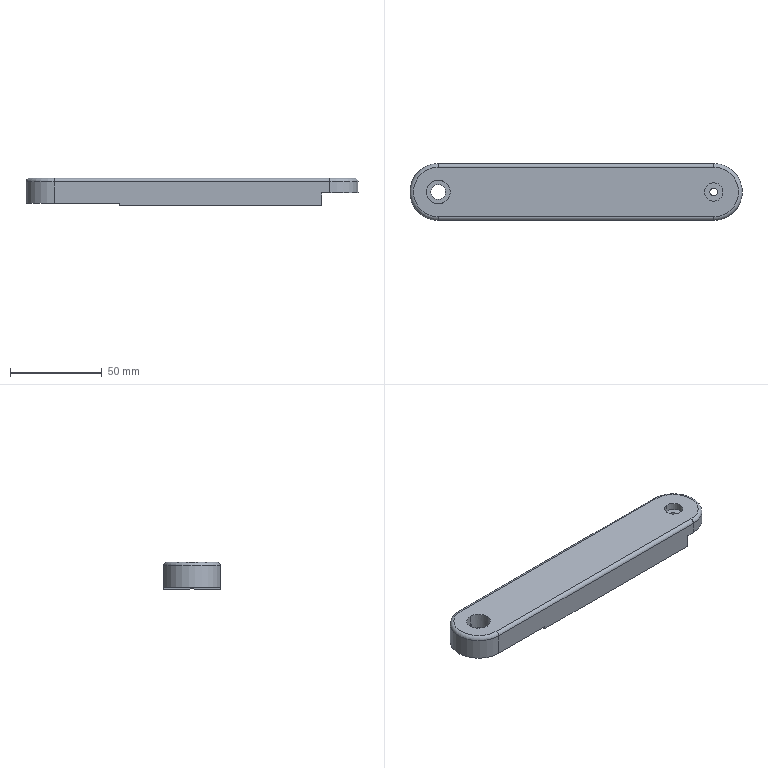NC program | NX | posted with a generic post | part box 181 x 31 x 15 mm
Lines 1 to 1656 of 2910:
N10 G17 G21 G94 G90
(FLOOR_WALL_COPY , TOOL : D80)
N12 T19 M6
N14 G54
N16 G17 G0 G90 X-138.5 Y0. S6500 M3
N18 G43 Z30. H19
N20 Z3.
N22 G94 G1 Z0. F1500.
N24 X-133.5
N26 X133.5
N28 X138.5
N30 Z3.
N32 G0 Z30.
N34 M5
(DRILLING_COPY_1 , TOOL : D6A45)
N36 T01 M6
N38 G54
N40 G17 G0 G90 X-79.5 Y7.794 S5000 M3
N42 G43 Z30. H1
N44 G94 G81 G98 Z-1. F350. R3.
N46 X-75. Y0.
N48 X-70.5 Y-7.794
N50 X43. Y-12.5
N52 X61.
N54 X75. Y0.
N56 X61. Y12.5
N58 X43.
N60 G80
N62 G0 X43. Y12.5 Z30.
N64 M5
(DRILLING_COPY_1_COPY , TOOL : 2.1ZT)
N66 T02 M6
N68 G54
N70 G17 G0 G90 X-79.5 Y7.794 S2000 M3
N72 G43 Z30. H2
N74 G94 G83 G98 Z-13.616 F150. Q2. R3.
N76 X-70.5 Y-7.794
N78 G80
N80 G0 X-70.5 Y-7.794 Z30.
N82 M5
(DRILLING_COPY_1_COPY_COPY , TOOL : 1.6ZT)
N84 T16 M6
N86 G54
N88 G17 G0 G90 X61. Y-12.5 S2000 M3
N90 G43 Z30. H16
N92 G94 G83 G98 Z-6.981 F150. Q2. R3.
N94 X43.
N96 Y12.5
N98 X61.
N100 G80
N102 G0 X61. Y12.5 Z30.
N104 M5
(DRILLING_COPY_1_COPY_COPY_COPY , TOOL : 1.5ZT)
N106 T24 M6
N108 G54
N110 G17 G0 G90 X61. Y-12.5 S2000 M3
N112 G43 Z30. H24
N114 G94 G83 G98 Z-9.751 F150. Q2. R3.
N116 X43.
N118 Y12.5
N120 X61.
N122 G80
N124 G0 X61. Y12.5 Z30.
N126 M5
(DRILLING_COPY_1_COPY_1 , TOOL : 4.2ZT)
N128 T04 M6
N130 G54
N132 G17 G0 G90 X-75. Y0. S2000 M3
N134 G43 Z30. H4
N136 G94 G83 G98 Z-17.262 F200. Q2. R3.
N138 G80
N140 G0 X-75. Y0. Z30.
N142 M5
(ADAPTIVE_MILLING , TOOL : D10)
N144 T15 M6
N146 G54
N148 G17 G0 G90 X-101.27 Y0.814 S9500 M3
N150 G43 Z30. H15
N152 Z-12.
N154 G94 G1 Z-15. F1000.
N156 X-99.799 Y0.354 F3000.
N158 G3 X-98.623 Y0.814 R1.017
N160 X-97.841 Y3.611 R6.974
N162 X-97.524 Y12.226 R84.168
N164 G2 X-97.472 Y16.099 R67.119
N166 X-94.519 Y20.246 R6.147
N168 X-88.73 Y22.087 R13.961
N170 X-79.743 Y22.468 R81.436
N172 G1 X-78.243 Y22.476
N174 X-76.243 Y22.482
N176 X-73.243 Y22.486
N178 X-66.868 Y22.487
N180 X90.507 Y22.488
N182 X90.632 Y22.486
N184 G2 X94.908 Y19.982 R5.724
N186 X96.946 Y14.663 R12.198
N188 X97.453 Y6.436 R56.701
N190 G1 X97.464 Y5.311
N192 X97.472 Y4.061
N194 X97.479 Y2.436
N196 X97.483 Y0.186
N198 X97.486 Y-3.564
N200 X97.487 Y-15.564
N202 G2 X95.036 Y-19.869 R5.707
N204 X89.483 Y-21.977 R12.35
N206 X80.879 Y-22.459 R62.316
N208 G1 X79.879 Y-22.468
N210 X78.504 Y-22.475
N212 X76.629 Y-22.481
N214 X73.879 Y-22.485
N216 X68.379 Y-22.487
N218 X-90.496 Y-22.488
N220 X-90.621 Y-22.486
N222 X-90.746 Y-22.48
N224 X-90.871 Y-22.47
N226 G2 X-95.119 Y-19.682 R5.969
N228 X-97.02 Y-14.176 R13.106
N230 X-97.461 Y-5.569 R68.61
N232 X-97.066 Y1.66 R38.858
N234 G3 X-96.535 Y12.892 R111.172
N236 G2 X-92.635 Y18.959 R7.799
N238 X-86.13 Y21.015 R16.183
N240 X-76.395 Y21.452 R87.612
N242 G1 X-75.02 Y21.461
N244 X-73.27 Y21.468
N246 X-70.77 Y21.473
N248 X-66.645 Y21.476
N250 X-53.27 Y21.477
N252 X87.355
N254 G2 X93.741 Y17.927 R7.581
N256 X95.923 Y11.729 R15.055
N258 X96.438 Y2.751 R67.51
N260 X96.445 Y-13.123 R725.539
N262 X92.701 Y-18.888 R7.731
N264 X86.463 Y-20.964 R15.603
N266 X77.607 Y-21.441 R72.154
N268 G1 X76.482 Y-21.451
N270 X75.107 Y-21.46
N272 X73.482 Y-21.467
N274 X71.107 Y-21.472
N276 X67.232 Y-21.476
N278 X56.232 Y-21.477
N280 X-87.393
N282 X-87.518 Y-21.476
N284 X-87.643 Y-21.474
N286 X-87.768 Y-21.469
N288 X-87.893 Y-21.463
N290 G2 X-93.897 Y-17.684 R7.684
N292 X-95.984 Y-11.319 R15.814
N294 X-96.087 Y0.903 R52.925
N296 G3 X-95.569 Y10.763 R219.063
N298 G2 X-90.669 Y18.005 R9.085
N300 X-83.747 Y20.004 R18.791
N302 X-78.228 Y20.365 R73.9
N304 G1 X-77.612 Y20.482
N306 X-77.546 Y20.49
N308 X-75.017 Y20.649
N310 X-74.983 Y20.65
N312 X74.983
N314 X75.017 Y20.649
N316 G3 X85.264 Y20.48 R204.238
N318 G2 X92.823 Y15.904 R8.884
N320 X94.976 Y8.905 R17.958
N322 X95.36 Y3.365 R66.902
N324 G1 X95.63 Y0.869
N326 X95.632 Y0.821
N328 G3 X95.459 Y-10.643 R652.19
N330 G2 X90.684 Y-17.955 R8.96
N332 X83.899 Y-19.977 R18.362
N334 X78.257 Y-20.364 R69.374
N336 G1 X77.8 Y-20.457
N338 X77.729 Y-20.466
N340 X75.018 Y-20.649
N342 X74.982 Y-20.65
N344 X-74.982
N346 X-75.018 Y-20.649
N348 G3 X-85.265 Y-20.48 R220.863
N350 G2 X-92.888 Y-15.795 R8.923
N352 X-94.975 Y-8.903 R18.027
N354 X-95.255 Y-3.811 R39.319
N356 G1 X-95.554 Y-1.965
N358 X-95.561 Y-1.894
N360 X-95.632 Y0.821
N362 X-95.63 Y0.869
N364 G2 X-94.998 Y5.602 R63.089
N366 X-94.523 Y9.949 R58.421
N368 X-88.915 Y17.045 R10.163
N370 X-83.574 Y18.742 R19.775
N372 X-78.121 Y20.385 R18.909
N374 G3 X-78.179 Y22.359 R1.
N376 G1 X-80.172 Y22.531 Z-14.9
N378 X-81.69 Y22.661
N380 X-81.855 Y22.658
N382 X-82.018 Y22.635
N384 X-83.654 Y22.228
N386 X-85.278 Y21.775
N388 X-86.341 Y21.412
N390 X-87.389 Y21.01
N392 X-90.269 Y19.806
N394 G3 X-94.133 Y17.169 R13.759
N396 X-97.045 Y12.184 R11.227
N398 G1 X-98.508 Y6.812
N400 G3 X-98.45 Y6.128 R1.033
N402 G1 X-97.699 Y4.513
N404 X-97.421 Y3.904 Z-14.934
N406 X-97.122 Y3.305 Z-14.967
N408 G3 X-96.601 Y2.918 Z-15. R1.041
N410 X-95.326 Y3.63 R1.004
N412 G2 X-93.357 Y10.099 R45.319
N414 X-88.93 Y15.227 R11.482
N416 X-84.888 Y18.127 R23.264
N418 G1 X-83.529 Y18.763
N420 G3 X-84.812 Y20.497 R-1.1
N422 G1 X-96.403 Y7.694
N424 G3 X-94.565 Y6.552 R-1.1
N426 G2 X-92.378 Y11.15 R22.853
N428 X-88.879 Y15.269 R22.812
N430 G3 X-89.472 Y17.04 R1.001
N432 X-90.087 Y16.883 Z-14.968 R1.328
N434 G1 X-91.335 Y16.348 Z-14.9
N436 X-92.2 Y15.983
N438 X-93.056 Y15.596
N440 X-93.234 Y15.449
N442 X-93.379 Y15.269
N444 X-95.453 Y11.833
N446 G3 X-97.872 Y6.327 R29.477
N448 X-98.638 Y0.906 R17.669
N450 G1 X-98.594 Y-1.815
N452 X-98.533 Y-4.536
N454 G3 X-97.734 Y-10.888 R39.929
N456 X-96.937 Y-14.175 R32.486
N458 X-95.435 Y-17.803 R24.395
N460 X-92.957 Y-20.719 R9.222
N462 X-89.002 Y-22.949 R15.307
N464 X-87.402 Y-23.323 R8.008
N466 G1 X-86.163 Y-23.447
N468 X-84.92 Y-23.528
N470 X-78.823 Y-23.789
N472 X-78.619 Y-23.773
N474 X-78.421 Y-23.723
N476 X-76.694 Y-23.057
N478 X-75.222 Y-22.479 Z-14.979
N480 X-75.054 Y-22.356 Z-14.99
N482 X-74.909 Y-22.206 Z-15.
N484 G3 X-75.641 Y-20.607 R1.002
N486 G1 X-77.729 Y-20.466
N488 X-77.8 Y-20.457
N490 G3 X-83.978 Y-19.568 R37.155
N492 G2 X-92.004 Y-13.916 R10.122
N494 X-93.713 Y-8.621 R18.894
N496 G1 X-94.296 Y-7.349
N498 X-94.321 Y-7.282
N500 X-95.106 Y-4.699
N502 X-95.122 Y-4.63
N504 X-95.262 Y-3.766
N506 G3 X-97.223 Y-3.701 R1.
N508 G1 X-97.324 Y-4.696 Z-14.95
N510 X-97.408 Y-5.692 Z-14.9
N512 X-97.552 Y-7.416
N514 X-97.512 Y-7.663
N516 G3 X-96.098 Y-12.12 R69.932
N518 G1 X-95.503 Y-13.665
N520 X-94.889 Y-15.203
N522 G3 X-92.265 Y-18.784 R10.103
N524 G1 X-91.374 Y-19.547
N526 X-90.451 Y-20.272
N528 G3 X-87.034 Y-21.984 R12.571
N530 G1 X-83.431 Y-23.139
N532 G3 X-82.703 Y-23.092 R1.03
N534 G1 X-81.102 Y-22.345
N536 X-80.489 Y-22.064 Z-14.934
N538 X-79.885 Y-21.762 Z-14.968
N540 G3 X-79.5 Y-21.252 Z-15. R1.042
N542 X-80.249 Y-19.957 R1.004
N544 G2 X-85.109 Y-18.275 R72.404
N546 X-90.065 Y-14.1 R11.496
N548 G1 X-91.654 Y-12.206
N550 X-91.696 Y-12.148
N552 X-93.138 Y-9.866
N554 X-93.172 Y-9.803
N556 X-93.744 Y-8.553
N558 G3 X-95.501 Y-9.81 R-1.1
N560 G1 X-83.638 Y-21.035
N562 G3 X-82.52 Y-19.198 R-1.1
N564 G1 X-83.063 Y-19.008
N566 X-83.128 Y-18.981
N568 X-85.535 Y-17.758
N570 X-85.596 Y-17.721
N572 X-87.818 Y-16.187
N574 X-87.873 Y-16.143
N576 G2 X-90.08 Y-14.083 R37.016
N578 G3 X-91.809 Y-14.404 R1.012
N580 G1 X-92.011 Y-14.981
N582 X-92.193 Y-15.565
N584 G3 X-90.958 Y-16.714 R1.012
N586 G1 Z-12.
N588 G0 Z30.
N590 X72.905 Y23.15
N592 Z-12.
N594 G1 Z-15. F1000.
N596 G2 X73.956 Y22.768 R1.02 F3000.
N598 G1 X74.649 Y21.819
N600 X75.361 Y20.883
N602 G3 X76.015 Y20.586 R1.041
N604 G1 X77.546 Y20.49
N606 X77.612 Y20.482
N608 G3 X84.183 Y19.547 R47.705
N610 G2 X92.039 Y13.847 R10.124
N612 X93.675 Y8.804 R18.58
N614 G1 X94.657 Y6.319
N616 X94.679 Y6.251
N618 G2 X95.365 Y3.312 R37.016
N620 G3 X97.331 Y3.18 R1.
N622 G1 X97.43 Y4.126 Z-14.952
N624 X97.503 Y5.075 Z-14.905
N626 X97.511 Y5.171 Z-14.9
N628 X97.656 Y6.965
N630 X97.615 Y7.209
N632 G3 X96.202 Y11.666 R69.932
N634 G1 X95.696 Y12.977
N636 X95.175 Y14.283
N638 G3 X92.922 Y17.991 R15.816
N640 X90.668 Y20.12 R14.524
N642 X86.313 Y22.355 R12.095
N644 G1 X83.268 Y23.194
N646 G3 X82.578 Y23.135 R1.033
N648 G1 X80.963 Y22.379
N650 X80.359 Y22.102 Z-14.933
N652 X79.765 Y21.803 Z-14.967
N654 G3 X79.377 Y21.272 Z-15. R1.04
N656 X80.086 Y20.012 R1.004
N658 G2 X85.357 Y18.18 R51.041
N660 X90.163 Y13.96 R11.634
N662 G1 X90.849 Y13.234
N664 X90.892 Y13.183
N666 G2 X93.71 Y8.715 R23.235
N668 G3 X95.488 Y9.919 R-1.1
N670 G1 X83.705 Y21.043
N672 G3 X82.546 Y19.22 R-1.1
N674 G2 X89.121 Y15.065 R22.222
N676 G1 X90.236 Y13.883
N678 X90.892 Y13.183
N680 G2 X93.664 Y8.831 R24.101
N682 G1 X94.679 Y6.251
N684 X95.338 Y3.56
N686 X95.632 Y0.821
N688 X95.561 Y-1.894
N690 G3 X94.784 Y-6.671 R193.406
N692 G2 X94.19 Y-10.871 R21.676
N694 X88.531 Y-17.198 R10.306
N696 X83.642 Y-18.719 R20.319
N698 G1 X83.128 Y-18.981
N700 X83.063 Y-19.008
N702 X80.514 Y-19.898
N704 X80.445 Y-19.917
N706 X78.24 Y-20.367
N708 G3 X78.229 Y-22.324 R1.
N710 G1 X80.22 Y-22.505 Z-14.9
N712 X81.808 Y-22.643
N714 X81.974 Y-22.639
N716 X82.138 Y-22.617
N718 X83.774 Y-22.21
N720 X85.398 Y-21.757
N722 G3 X90.332 Y-19.68 R29.809
N724 X93.391 Y-17.703 R27.075
N726 X97.153 Y-12.07 R10.652
N728 G1 X98.288 Y-7.881
N730 G3 X98.224 Y-7.187 R1.032
N732 G1 X97.463 Y-5.598
N734 X97.182 Y-4.999 Z-14.933
N736 X96.879 Y-4.412 Z-14.966
N738 G3 X96.337 Y-4.028 Z-15. R1.039
N740 X95.106 Y-4.699 R1.005
N742 G2 X93.164 Y-10.392 R44.823
N744 X88.927 Y-15.184 R11.629
N746 G1 X87.873 Y-16.143
N748 X87.818 Y-16.187
N750 X85.596 Y-17.721
N752 X85.535 Y-17.758
N754 X83.64 Y-18.72
N756 G3 X84.941 Y-20.453 R-1.1
N758 G1 X96.098 Y-8.559
N760 G3 X94.296 Y-7.349 R-1.1
N762 G1 X93.172 Y-9.803
N764 X93.138 Y-9.866
N766 X91.696 Y-12.148
N768 X91.654 Y-12.206
N770 X89.919 Y-14.274
N772 X89.87 Y-14.325
N774 X88.853 Y-15.251
N776 G3 X88.895 Y-16.781 R1.014
N778 G1 X89.946 Y-17.636
N780 Z-12.
N782 G0 Z30.
(FLOOR_WALL , TOOL : D10)
N784 X-97.071 Y-4.371
N786 Z0.014
N788 G1 Z-0.986 F1000.
N790 X-91. Y-0.866
N792 G3 X-90.5 Y0. R1.
N794 G2 X-75.79 Y15.48 R15.5 F2500.
N796 G3 X-71.991 Y10.216 R5.3
N798 G2 X-71.991 Y-10.216 R10.65
N800 G3 X-75.79 Y-15.48 R5.3
N802 G2 X-90.5 Y0. R15.5
N804 G1 X-85.5
N806 G2 X-79.112 Y9.661 R10.5
N808 G3 X-73.403 Y5.42 R10.3
N810 G2 X-73.403 Y-5.42 R5.65
N812 G3 X-79.112 Y-9.661 R10.3
N814 G2 X-85.5 Y0. R10.5
N816 G1 X-80.5
N818 G2 X-79.604 Y3.009 R5.5
N820 G3 X-74.816 Y0.624 R15.3
N822 G2 X-74.816 Y-0.624 R0.65
N824 G3 X-79.604 Y-3.009 R15.3
N826 G2 X-80.5 Y0. R5.5
N828 G3 X-81. Y0.866 R1.
N830 G1 Z0.014
N832 G0 X-97.071 Y-4.371 Z-0.971
N834 G1 Z-1.971 F1000.
N836 X-91. Y-0.866
N838 G3 X-90.5 Y0. R1.
N840 G2 X-75.79 Y15.48 R15.5 F2500.
N842 G3 X-71.991 Y10.216 R5.3
N844 G2 X-71.991 Y-10.216 R10.65
N846 G3 X-75.79 Y-15.48 R5.3
N848 G2 X-90.5 Y0. R15.5
N850 G1 X-85.5
N852 G2 X-79.112 Y9.661 R10.5
N854 G3 X-73.403 Y5.42 R10.3
N856 G2 X-73.403 Y-5.42 R5.65
N858 G3 X-79.112 Y-9.661 R10.3
N860 G2 X-85.5 Y0. R10.5
N862 G1 X-80.5
N864 G2 X-79.604 Y3.009 R5.5
N866 G3 X-74.816 Y0.624 R15.3
N868 G2 X-74.816 Y-0.624 R0.65
N870 G3 X-79.604 Y-3.009 R15.3
N872 G2 X-80.5 Y0. R5.5
N874 G3 X-81. Y0.866 R1.
N876 G1 Z-0.971
N878 G0 X-97.071 Y-4.371 Z-1.957
N880 G1 Z-2.957 F1000.
N882 X-91. Y-0.866
N884 G3 X-90.5 Y0. R1.
N886 G2 X-75.79 Y15.48 R15.5 F2500.
N888 G3 X-71.991 Y10.216 R5.3
N890 G2 X-71.991 Y-10.216 R10.65
N892 G3 X-75.79 Y-15.48 R5.3
N894 G2 X-90.5 Y0. R15.5
N896 G1 X-85.5
N898 G2 X-79.112 Y9.661 R10.5
N900 G3 X-73.403 Y5.42 R10.3
N902 G2 X-73.403 Y-5.42 R5.65
N904 G3 X-79.112 Y-9.661 R10.3
N906 G2 X-85.5 Y0. R10.5
N908 G1 X-80.5
N910 G2 X-79.604 Y3.009 R5.5
N912 G3 X-74.816 Y0.624 R15.3
N914 G2 X-74.816 Y-0.624 R0.65
N916 G3 X-79.604 Y-3.009 R15.3
N918 G2 X-80.5 Y0. R5.5
N920 G3 X-81. Y0.866 R1.
N922 G1 Z-1.957
N924 G0 X-97.071 Y-4.371 Z-2.943
N926 G1 Z-3.943 F1000.
N928 X-91. Y-0.866
N930 G3 X-90.5 Y0. R1.
N932 G2 X-75.79 Y15.48 R15.5 F2500.
N934 G3 X-71.991 Y10.216 R5.3
N936 G2 X-71.991 Y-10.216 R10.65
N938 G3 X-75.79 Y-15.48 R5.3
N940 G2 X-90.5 Y0. R15.5
N942 G1 X-85.5
N944 G2 X-79.112 Y9.661 R10.5
N946 G3 X-73.403 Y5.42 R10.3
N948 G2 X-73.403 Y-5.42 R5.65
N950 G3 X-79.112 Y-9.661 R10.3
N952 G2 X-85.5 Y0. R10.5
N954 G1 X-80.5
N956 G2 X-79.604 Y3.009 R5.5
N958 G3 X-74.816 Y0.624 R15.3
N960 G2 X-74.816 Y-0.624 R0.65
N962 G3 X-79.604 Y-3.009 R15.3
N964 G2 X-80.5 Y0. R5.5
N966 G3 X-81. Y0.866 R1.
N968 G1 Z-2.943
N970 G0 X-97.071 Y-4.371 Z-3.929
N972 G1 Z-4.929 F1000.
N974 X-91. Y-0.866
N976 G3 X-90.5 Y0. R1.
N978 G2 X-75.79 Y15.48 R15.5 F2500.
N980 G3 X-71.991 Y10.216 R5.3
N982 G2 X-71.991 Y-10.216 R10.65
N984 G3 X-75.79 Y-15.48 R5.3
N986 G2 X-90.5 Y0. R15.5
N988 G1 X-85.5
N990 G2 X-79.112 Y9.661 R10.5
N992 G3 X-73.403 Y5.42 R10.3
N994 G2 X-73.403 Y-5.42 R5.65
N996 G3 X-79.112 Y-9.661 R10.3
N998 G2 X-85.5 Y0. R10.5
N1000 G1 X-80.5
N1002 G2 X-79.604 Y3.009 R5.5
N1004 G3 X-74.816 Y0.624 R15.3
N1006 G2 X-74.816 Y-0.624 R0.65
N1008 G3 X-79.604 Y-3.009 R15.3
N1010 G2 X-80.5 Y0. R5.5
N1012 G3 X-81. Y0.866 R1.
N1014 G1 Z-3.929
N1016 G0 X-97.071 Y-4.371 Z-4.914
N1018 G1 Z-5.914 F1000.
N1020 X-91. Y-0.866
N1022 G3 X-90.5 Y0. R1.
N1024 G2 X-75.79 Y15.48 R15.5 F2500.
N1026 G3 X-71.991 Y10.216 R5.3
N1028 G2 X-71.991 Y-10.216 R10.65
N1030 G3 X-75.79 Y-15.48 R5.3
N1032 G2 X-90.5 Y0. R15.5
N1034 G1 X-85.5
N1036 G2 X-79.112 Y9.661 R10.5
N1038 G3 X-73.403 Y5.42 R10.3
N1040 G2 X-73.403 Y-5.42 R5.65
N1042 G3 X-79.112 Y-9.661 R10.3
N1044 G2 X-85.5 Y0. R10.5
N1046 G1 X-80.5
N1048 G2 X-79.604 Y3.009 R5.5
N1050 G3 X-74.816 Y0.624 R15.3
N1052 G2 X-74.816 Y-0.624 R0.65
N1054 G3 X-79.604 Y-3.009 R15.3
N1056 G2 X-80.5 Y0. R5.5
N1058 G3 X-81. Y0.866 R1.
N1060 G1 Z-4.914
N1062 G0 X-97.071 Y-4.371 Z-5.9
N1064 G1 Z-6.9 F1000.
N1066 X-91. Y-0.866
N1068 G3 X-90.5 Y0. R1.
N1070 G2 X-75.79 Y15.48 R15.5 F2500.
N1072 G3 X-71.991 Y10.216 R5.3
N1074 G2 X-71.991 Y-10.216 R10.65
N1076 G3 X-75.79 Y-15.48 R5.3
N1078 G2 X-90.5 Y0. R15.5
N1080 G1 X-85.5
N1082 G2 X-79.112 Y9.661 R10.5
N1084 G3 X-73.403 Y5.42 R10.3
N1086 G2 X-73.403 Y-5.42 R5.65
N1088 G3 X-79.112 Y-9.661 R10.3
N1090 G2 X-85.5 Y0. R10.5
N1092 G1 X-80.5
N1094 G2 X-79.604 Y3.009 R5.5
N1096 G3 X-74.816 Y0.624 R15.3
N1098 G2 X-74.816 Y-0.624 R0.65
N1100 G3 X-79.604 Y-3.009 R15.3
N1102 G2 X-80.5 Y0. R5.5
N1104 G3 X-81. Y0.866 R1.
N1106 G1 Z-5.9
N1108 G0 Z30.
(FLOOR_WALL_COPY_1 , TOOL : D10)
N1110 X97.283 Y3.068
N1112 Z0.4
N1114 G1 Z-0.6 F1000.
N1116 X90.997 Y-0.071
N1118 G3 X90.445 Y-0.906 R1.
N1120 G2 X75. Y-15.5 R15.443 F2500.
N1122 G1 X44.6
N1124 Y15.5
N1126 X75.
N1128 G2 X90.445 Y-0.906 R15.459
N1130 G1 X85.454 Y-0.604
N1132 G2 X74.849 Y-10.5 R10.469
N1134 G1 X49.6
N1136 Y10.5
N1138 X74.849
N1140 G2 X85.454 Y-0.604 R10.475
N1142 G1 X80.463 Y-0.302
N1144 G2 X74.698 Y-5.5 R5.503
N1146 G1 X54.6
N1148 Y5.5
N1150 X74.698
N1152 G2 X80.463 Y-0.302 R5.504
N1154 G1 X75.473 Y0.
N1156 X75.389 Y-0.268
N1158 X75.168 Y-0.442
N1160 X74.547 Y-0.5
N1162 X59.6
N1164 Y0.5
N1166 X74.547
N1168 X75.057 Y0.469
N1170 X75.313 Y0.354
N1172 X75.459 Y0.113
N1174 X75.469 Y0.057
N1176 X75.473 Y0.
N1178 G3 X76.024 Y-0.834 R1.
N1180 G1 Z0.4
N1182 G0 X97.283 Y3.068 Z-0.2
N1184 G1 Z-1.2 F1000.
N1186 X90.997 Y-0.071
N1188 G3 X90.445 Y-0.906 R1.
N1190 G2 X75. Y-15.5 R15.443 F2500.
N1192 G1 X44.6
N1194 Y15.5
N1196 X75.
N1198 G2 X90.445 Y-0.906 R15.459
N1200 G1 X85.454 Y-0.604
N1202 G2 X74.849 Y-10.5 R10.469
N1204 G1 X49.6
N1206 Y10.5
N1208 X74.849
N1210 G2 X85.454 Y-0.604 R10.475
N1212 G1 X80.463 Y-0.302
N1214 G2 X74.698 Y-5.5 R5.503
N1216 G1 X54.6
N1218 Y5.5
N1220 X74.698
N1222 G2 X80.463 Y-0.302 R5.504
N1224 G1 X75.473 Y0.
N1226 X75.389 Y-0.268
N1228 X75.168 Y-0.442
N1230 X74.547 Y-0.5
N1232 X59.6
N1234 Y0.5
N1236 X74.547
N1238 X75.057 Y0.469
N1240 X75.313 Y0.354
N1242 X75.459 Y0.113
N1244 X75.469 Y0.057
N1246 X75.473 Y0.
N1248 G3 X76.024 Y-0.834 R1.
N1250 G1 Z-0.2
N1252 G0 Z30.
N1254 M5
(ZLEVEL_PROFILE_COPY_1_COPY_COPY_1 , TOOL : D10JING)
N1256 T14 M6
N1258 G54
N1260 G17 G0 G90 X76.695 Y-22.436 S9500 M3
N1262 G43 Z30. H14
N1264 Z-14.
N1266 G94 G1 Z-15. F1000.
N1268 X75.866 Y-21.
N1270 G3 X75. Y-20.5 R1.
N1272 G1 X-75. F1200.
N1274 G2 X-95.5 Y0. R20.5
N1276 X-75. Y20.5 R20.5
N1278 G1 X75.
N1280 G2 X95.5 Y0. R20.5
N1282 X75. Y-20.5 R20.5
N1284 G3 X74.134 Y-21. R1.
N1286 G1 X73.268 Y-22.5
N1288 Z-14.
N1290 G0 Z30.
(FLOOR_WALL_1 , TOOL : D10JING)
N1292 X98.431 Y-1.389
N1294 Z1.7
N1296 G1 Z-1.3 F1250.
N1298 X90.445 Y-0.906
N1300 G2 X75. Y-15.5 R15.443
N1302 G1 X45.
N1304 Y15.5
N1306 X75.
N1308 G2 X90.445 Y-0.906 R15.454
N1310 G1 X85.454 Y-0.604
N1312 G2 X74.849 Y-10.5 R10.469
N1314 G1 X50.
N1316 Y10.5
N1318 X74.849
N1320 G2 X85.454 Y-0.604 R10.475
N1322 G1 X80.463 Y-0.302
N1324 G2 X74.698 Y-5.5 R5.503
N1326 G1 X55.
N1328 Y5.5
N1330 X74.698
N1332 G2 X80.463 Y-0.302 R5.504
N1334 G1 X75.473 Y0.
N1336 X75.389 Y-0.268
N1338 X75.168 Y-0.442
N1340 X74.547 Y-0.5
N1342 X60.
N1344 Y0.5
N1346 X74.547
N1348 X75.057 Y0.469
N1350 X75.313 Y0.354
N1352 X75.459 Y0.113
N1354 X75.469 Y0.057
N1356 X75.473 Y0.
N1358 X78.467 Y0.181
N1360 Z1.7
N1362 G0 Z30.
N1364 X44.5 Y23.5
N1366 Z1.7
N1368 G1 Z-1.3
N1370 Y15.5
N1372 Y-15.5
N1374 Y-23.5
N1376 Z1.7
N1378 G0 Z30.
N1380 X-98.449 Y1.087
N1382 Z-4.
N1384 G1 Z-7.
N1386 X-90.463 Y0.604
N1388 G2 X-76.192 Y15.428 R15.4
N1390 G3 X-72.104 Y9.832 R5.7
N1392 G2 X-72.104 Y-9.832 R10.25
N1394 G3 X-76.192 Y-15.428 R5.7
N1396 G1 X-76.868 Y-15.387
N1398 G2 X-90.463 Y0.604 R15.454
N1400 G1 X-85.473 Y0.302
N1402 G2 X-79.467 Y9.473 R10.385
N1404 G3 X-73.517 Y5.036 R10.7
N1406 G2 X-73.517 Y-5.036 R5.25
N1408 G3 X-79.467 Y-9.473 R10.7
N1410 G2 X-85.473 Y0.302 R10.394
N1412 G1 X-80.482 Y0.
N1414 G2 X-79.792 Y2.65 R5.394
N1416 G3 X-74.929 Y0.24 R15.7
N1418 G2 X-74.929 Y-0.24 R0.25
N1420 G3 X-79.792 Y-2.65 R15.7
N1422 G2 X-80.482 Y0. R5.323
N1424 G1 X-83.476 Y-0.181
N1426 Z-4.
N1428 G0 Z30.
N1430 X-75.447 Y-23.455
N1432 Z-4.
N1434 G1 Z-7.
N1436 X-75.691 Y-15.458
N1438 G2 X-71.962 Y-10.312 R5.2
N1440 G3 X-71.962 Y10.312 R10.75
N1442 G2 X-75.691 Y15.458 R5.2
N1444 G1 X-75.447 Y23.455
N1446 Z-4.
N1448 G0 Z30.
N1450 M5
(FLOOR_WALL_COPY_1_COPY , TOOL : D6)
N1452 T12 M6
N1454 G54
N1456 G17 G0 G90 X48.6 Y0.14 S9500 M3
N1458 G43 Z30. H12
N1460 Z-0.3
N1462 G94 G1 Y-0.9 Z-0.355 F1000.
N1464 X60.4 Z-0.973
N1466 Y0.9 Z-1.067
N1468 X48.6 Z-1.686
N1470 Y-0.9 Z-1.78
N1472 X60.4 F1650.
N1474 Y0.9
N1476 X48.6
N1478 Y-0.9
N1480 X45.6
N1482 Y-3.9
N1484 X62.5
N1486 G2 X63.4 Y-3.957 R7.1
N1488 G1 Y3.957
N1490 G2 X62.5 Y3.9 R7.1
N1492 G1 X45.6
N1494 Y-0.9
N1496 X42.6
N1498 Y-6.9
N1500 X62.5
N1502 G2 X66.6 Y-11. R4.1
N1504 G1 Y-11.7
N1506 X74.427
N1508 X74.439 Y-11.673
N1510 G2 X74.439 Y-9.327 R1.3
N1512 G1 X74.427 Y-9.3
N1514 X70.5
N1516 G2 X66.4 Y-5.2 R4.1
N1518 G1 Y5.2
N1520 G2 X70.5 Y9.3 R4.1
N1522 G1 X74.427
N1524 X74.439 Y9.327
N1526 G2 X74.439 Y11.673 R1.3
N1528 G1 X74.427 Y11.7
N1530 X66.6
N1532 Y11.
N1534 G2 X62.5 Y6.9 R4.1
N1536 G1 X42.6
N1538 Y-0.9
N1540 Z-0.78
N1542 G0 X48.6 Y0.14
N1544 G1 Y-0.9 Z-0.835 F1000.
N1546 X60.4 Z-1.453
N1548 Y0.9 Z-1.547
N1550 X48.6 Z-2.166
N1552 Y-0.9 Z-2.26
N1554 X60.4 F1650.
N1556 Y0.9
N1558 X48.6
N1560 Y-0.9
N1562 X45.6
N1564 Y-3.9
N1566 X62.5
N1568 G2 X63.4 Y-3.957 R7.1
N1570 G1 Y3.957
N1572 G2 X62.5 Y3.9 R7.1
N1574 G1 X45.6
N1576 Y-0.9
N1578 X42.6
N1580 Y-6.9
N1582 X62.5
N1584 G2 X66.6 Y-11. R4.1
N1586 G1 Y-11.7
N1588 X74.427
N1590 X74.439 Y-11.673
N1592 G2 X74.439 Y-9.327 R1.3
N1594 G1 X74.427 Y-9.3
N1596 X70.5
N1598 G2 X66.4 Y-5.2 R4.1
N1600 G1 Y5.2
N1602 G2 X70.5 Y9.3 R4.1
N1604 G1 X74.427
N1606 X74.439 Y9.327
N1608 G2 X74.439 Y11.673 R1.3
N1610 G1 X74.427 Y11.7
N1612 X66.6
N1614 Y11.
N1616 G2 X62.5 Y6.9 R4.1
N1618 G1 X42.6
N1620 Y-0.9
N1622 Z-1.26
N1624 G0 X48.6 Y0.14
N1626 G1 Y-0.9 Z-1.315 F1000.
N1628 X60.4 Z-1.933
N1630 Y0.9 Z-2.027
N1632 X48.6 Z-2.646
N1634 Y-0.9 Z-2.74
N1636 X60.4 F1650.
N1638 Y0.9
N1640 X48.6
N1642 Y-0.9
N1644 X45.6
N1646 Y-3.9
N1648 X62.5
N1650 G2 X63.4 Y-3.957 R7.1
N1652 G1 Y3.957
N1654 G2 X62.5 Y3.9 R7.1
N1656 G1 X45.6
N1658 Y-0.9
N1660 X42.6
N1662 Y-6.9
N1664 X62.5
N1666 G2 X66.6 Y-11. R4.1
N1668 G1 Y-11.7
N1670 X74.427
N1672 X74.439 Y-11.673
N1674 G2 X74.439 Y-9.327 R1.3
N1676 G1 X74.427 Y-9.3
N1678 X70.5
N1680 G2 X66.4 Y-5.2 R4.1
N1682 G1 Y5.2
N1684 G2 X70.5 Y9.3 R4.1
N1686 G1 X74.427
N1688 X74.439 Y9.327
N1690 G2 X74.439 Y11.673 R1.3
N1692 G1 X74.427 Y11.7
N1694 X66.6
N1696 Y11.
N1698 G2 X62.5 Y6.9 R4.1
N1700 G1 X42.6
N1702 Y-0.9
N1704 Z-1.74
N1706 G0 X48.6 Y0.14
N1708 G1 Y-0.9 Z-1.795 F1000.
N1710 X60.4 Z-2.413
N1712 Y0.9 Z-2.507
N1714 X48.6 Z-3.126
N1716 Y-0.9 Z-3.22
N1718 X60.4 F1650.
N1720 Y0.9
N1722 X48.6
N1724 Y-0.9
N1726 X45.6
N1728 Y-3.9
N1730 X62.5
N1732 G2 X63.4 Y-3.957 R7.1
N1734 G1 Y3.957
N1736 G2 X62.5 Y3.9 R7.1
N1738 G1 X45.6
N1740 Y-0.9
N1742 X42.6
N1744 Y-6.9
N1746 X62.5
N1748 G2 X66.6 Y-11. R4.1
N1750 G1 Y-11.7
N1752 X74.427
N1754 X74.439 Y-11.673
N1756 G2 X74.439 Y-9.327 R1.3
N1758 G1 X74.427 Y-9.3
N1760 X70.5
N1762 G2 X66.4 Y-5.2 R4.1
N1764 G1 Y5.2
N1766 G2 X70.5 Y9.3 R4.1
N1768 G1 X74.427
N1770 X74.439 Y9.327
N1772 G2 X74.439 Y11.673 R1.3
N1774 G1 X74.427 Y11.7
N1776 X66.6
N1778 Y11.
N1780 G2 X62.5 Y6.9 R4.1
N1782 G1 X42.6
N1784 Y-0.9
N1786 Z-2.22
N1788 G0 X48.6 Y0.14
N1790 G1 Y-0.9 Z-2.275 F1000.
N1792 X60.4 Z-2.893
N1794 Y0.9 Z-2.987
N1796 X48.6 Z-3.606
N1798 Y-0.9 Z-3.7
N1800 X60.4 F1650.
N1802 Y0.9
N1804 X48.6
N1806 Y-0.9
N1808 X45.6
N1810 Y-3.9
N1812 X62.5
N1814 G2 X63.4 Y-3.957 R7.1
N1816 G1 Y3.957
N1818 G2 X62.5 Y3.9 R7.1
N1820 G1 X45.6
N1822 Y-0.9
N1824 X42.6
N1826 Y-6.9
N1828 X62.5
N1830 G2 X66.6 Y-11. R4.1
N1832 G1 Y-11.7
N1834 X74.427
N1836 X74.439 Y-11.673
N1838 G2 X74.439 Y-9.327 R1.3
N1840 G1 X74.427 Y-9.3
N1842 X70.5
N1844 G2 X66.4 Y-5.2 R4.1
N1846 G1 Y5.2
N1848 G2 X70.5 Y9.3 R4.1
N1850 G1 X74.427
N1852 X74.439 Y9.327
N1854 G2 X74.439 Y11.673 R1.3
N1856 G1 X74.427 Y11.7
N1858 X66.6
N1860 Y11.
N1862 G2 X62.5 Y6.9 R4.1
N1864 G1 X42.6
N1866 Y-0.9
N1868 Z-2.7
N1870 G0 Z30.
(FLOOR_WALL_1_COPY , TOOL : D6)
N1872 X66.057 Y8.622
N1874 Z-0.7
N1876 G1 X66.44 Y9.204 Z-0.887 F1250.
N1878 X66.8 Y10.491 Z-1.245
N1880 Y11.5 Z-1.515
N1882 X74.169 Z-3.49
N1884 X73.953 Y11.321 Z-3.565
N1886 X73.7 Y10.781 Z-3.725
N1888 Y10.5 Z-3.8
N1890 G3 X74.169 Y9.5 R1.3
N1892 G1 X70.5
N1894 G3 X66.2 Y5.2 R4.3
N1896 G1 Y-5.2
N1898 G3 X70.5 Y-9.5 R4.3
N1900 G1 X74.169
N1902 G3 X74.169 Y-11.5 R1.3
N1904 G1 X66.8
N1906 Y-11.
N1908 G3 X62.5 Y-6.7 R4.3
N1910 G1 X42.8
N1912 Y6.7
N1914 X62.5
N1916 G3 X62.912 Y6.72 R4.3
N1918 G1 X63.2 Y3.734
N1920 Y-3.734
N1922 G3 X62.5 Y-3.7 R7.3
N1924 G1 X45.8
N1926 Y3.7
N1928 X62.5
N1930 G3 X63.2 Y3.734 R7.3
N1932 G1 X60.2 Y0.7
N1934 Y-0.7
N1936 X48.8
N1938 Y0.7
N1940 X60.2
N1942 X63.2 Y3.734
N1944 X62.912 Y6.72
N1946 G3 X66.8 Y11. R4.3
N1948 G1 Y11.5
N1950 X74.169
N1952 G3 X73.7 Y10.5 R1.3
N1954 G1 X75.2
N1956 Z-0.8
N1958 G0 Z30.
N1960 X65.699 Y8.64
N1962 Z-0.7
N1964 G1 X66.122 Y9.234 Z-0.895
N1966 X66.5 Y10.509 Z-1.252
N1968 Y11.8 Z-1.598
N1970 X74.719 Z-3.8
N1972 X66.5
N1974 Y11.
N1976 G2 X62.5 Y7. R4.
N1978 G1 X42.5
N1980 Y-7.
N1982 X62.5
N1984 G2 X66.5 Y-11. R4.
N1986 G1 Y-11.8
N1988 X74.719
N1990 Z-0.8
N1992 G0 Z30.
N1994 Z-0.8
N1996 G1 Z-3.8
N1998 X74.725 Y-11.771
N2000 G2 X74.725 Y-9.229 R1.3
N2002 G1 X74.719 Y-9.2
N2004 X70.5
N2006 G2 X66.5 Y-5.2 R4.
N2008 G1 Y5.2
N2010 G2 X70.5 Y9.2 R4.
N2012 G1 X74.719
N2014 Z-0.8
N2016 G0 Z30.
(HOLE_MILLING , TOOL : D6)
N2018 X75. Y10.5
N2020 Z-0.8
N2022 G3 X74.4 Y11.1 R0.6 F1650.
N2024 X73.8 Y10.5 R0.6
N2026 X73.8 Y10.5 Z-1.3 I1.2 J0.
N2028 X73.8 Y10.5 Z-1.8 I1.2 J0.
N2030 X73.8 Y10.5 Z-2.3 I1.2 J0.
N2032 X73.8 Y10.5 Z-2.8 I1.2 J0.
N2034 X73.8 Y10.5 Z-3.3 I1.2 J0.
N2036 X73.8 Y10.5 Z-3.8 I1.2 J0.
N2038 X73.8 Y10.5 Z-4.3 I1.2 J0.
N2040 X73.8 Y10.5 Z-4.8 I1.2 J0.
N2042 X73.8 Y10.5 Z-5.3 I1.2 J0.
N2044 X73.8 Y10.5 Z-5.8 I1.2 J0.
N2046 X73.8 Y10.5 Z-6.3 I1.2 J0.
N2048 X73.8 Y10.5 Z-6.8 I1.2 J0.
N2050 X73.8 Y10.5 Z-7.3 I1.2 J0.
N2052 X73.8 Y10.5 Z-7.8 I1.2 J0.
N2054 X73.8 Y10.5 Z-8.3 I1.2 J0.
N2056 X73.8 Y10.5 Z-8.8 I1.2 J0.
N2058 X75.971 Y9.795 Z-9. R1.2
N2060 X75.705 Y11.471 R1.2
N2062 X75.971 Y9.795 R-1.2
N2064 X75.838 Y10.633 R0.6
N2066 X75. Y10.5 R0.6
N2068 G0 Z30.
N2070 Y-10.5
N2072 Z-0.8
N2074 G3 X74.4 Y-9.9 R0.6
N2076 X73.8 Y-10.5 R0.6
N2078 X73.8 Y-10.5 Z-1.3 I1.2 J0.
N2080 X73.8 Y-10.5 Z-1.8 I1.2 J0.
N2082 X73.8 Y-10.5 Z-2.3 I1.2 J0.
N2084 X73.8 Y-10.5 Z-2.8 I1.2 J0.
N2086 X73.8 Y-10.5 Z-3.3 I1.2 J0.
N2088 X73.8 Y-10.5 Z-3.8 I1.2 J0.
N2090 X73.8 Y-10.5 Z-4.3 I1.2 J0.
N2092 X73.8 Y-10.5 Z-4.8 I1.2 J0.
N2094 X73.8 Y-10.5 Z-5.3 I1.2 J0.
N2096 X73.8 Y-10.5 Z-5.8 I1.2 J0.
N2098 X73.8 Y-10.5 Z-6.3 I1.2 J0.
N2100 X73.8 Y-10.5 Z-6.8 I1.2 J0.
N2102 X73.8 Y-10.5 Z-7.3 I1.2 J0.
N2104 X73.8 Y-10.5 Z-7.8 I1.2 J0.
N2106 X73.8 Y-10.5 Z-8.3 I1.2 J0.
N2108 X73.8 Y-10.5 Z-8.8 I1.2 J0.
N2110 X75.971 Y-11.205 Z-9. R1.2
N2112 X75.705 Y-9.529 R1.2
N2114 X75.971 Y-11.205 R-1.2
N2116 X75.838 Y-10.367 R0.6
N2118 X75. Y-10.5 R0.6
N2120 G0 Z30.
N2122 M5
(HOLE_MILLING_COPY , TOOL : D4)
N2124 T11 M6
N2126 G54
N2128 G17 G0 G90 X75. Y0. S9500 M3
N2130 G43 Z30. H11
N2132 Z-0.8
N2134 G94 G3 X74.05 Y0.95 R0.95 F1650.
N2136 X73.1 Y0. R0.95
N2138 X73.1 Y0. Z-1.1 I1.9 J0.
N2140 X73.1 Y0. Z-1.4 I1.9 J0.
N2142 X73.1 Y0. Z-1.7 I1.9 J0.
N2144 X73.1 Y0. Z-2. I1.9 J0.
N2146 X73.1 Y0. Z-2.3 I1.9 J0.
N2148 X73.1 Y0. Z-2.6 I1.9 J0.
N2150 X73.1 Y0. Z-2.9 I1.9 J0.
N2152 X73.1 Y0. Z-3.2 I1.9 J0.
N2154 X73.1 Y0. Z-3.5 I1.9 J0.
N2156 X73.1 Y0. Z-3.8 I1.9 J0.
N2158 X73.1 Y0. Z-4.1 I1.9 J0.
N2160 X73.1 Y0. Z-4.4 I1.9 J0.
N2162 X73.1 Y0. Z-4.7 I1.9 J0.
N2164 X73.1 Y0. Z-5. I1.9 J0.
N2166 X73.1 Y0. Z-5.3 I1.9 J0.
N2168 X73.1 Y0. Z-5.6 I1.9 J0.
N2170 X73.1 Y0. Z-5.9 I1.9 J0.
N2172 X73.1 Y0. Z-6.2 I1.9 J0.
N2174 X73.1 Y0. Z-6.5 I1.9 J0.
N2176 X73.1 Y0. Z-6.8 I1.9 J0.
N2178 X73.1 Y0. Z-7.1 I1.9 J0.
N2180 X73.1 Y0. Z-7.4 I1.9 J0.
N2182 X73.1 Y0. Z-7.7 I1.9 J0.
N2184 X73.1 Y0. Z-8. I1.9 J0.
N2186 X73.1 Y0. Z-8.3 I1.9 J0.
N2188 X73.1 Y0. Z-8.6 I1.9 J0.
N2190 X73.1 Y0. Z-8.9 I1.9 J0.
N2192 X73.1 Y0. Z-9.2 I1.9 J0.
N2194 X73.1 Y0. Z-9.5 I1.9 J0.
N2196 X73.1 Y0. Z-9.8 I1.9 J0.
N2198 X73.1 Y0. Z-10.1 I1.9 J0.
N2200 X73.1 Y0. Z-10.4 I1.9 J0.
N2202 X73.1 Y0. Z-10.7 I1.9 J0.
N2204 X73.1 Y0. Z-11. I1.9 J0.
N2206 X73.1 Y0. Z-11.3 I1.9 J0.
N2208 X73.1 Y0. Z-11.6 I1.9 J0.
N2210 X73.1 Y0. Z-11.9 I1.9 J0.
N2212 X73.1 Y0. Z-12.2 I1.9 J0.
N2214 X73.1 Y0. Z-12.5 I1.9 J0.
N2216 X73.1 Y0. Z-12.8 I1.9 J0.
N2218 X73.1 Y0. Z-13.1 I1.9 J0.
N2220 X73.1 Y0. Z-13.4 I1.9 J0.
N2222 X73.1 Y0. Z-13.7 I1.9 J0.
N2224 X73.1 Y0. Z-14. I1.9 J0.
N2226 X73.1 Y0. Z-14.3 I1.9 J0.
N2228 X73.1 Y0. Z-14.6 I1.9 J0.
N2230 X73.1 Y0. Z-14.9 I1.9 J0.
N2232 X75.95 Y-1.645 Z-15. R1.9
N2234 X76.645 Y0.95 R1.9
N2236 X75.95 Y-1.645 R-1.9
N2238 X76.298 Y-0.348 R0.95
N2240 X75. Y0. R0.95
N2242 G0 Z30.
N2244 M5
(ZLEVEL_PROFILE , TOOL : D2)
N2246 T17 M6
N2248 G54
N2250 G17 G0 G90 X66.853 Y13.4 S9500 M3
N2252 G43 Z30. H17
N2254 Z-1.447
N2256 G94 G1 X66.68 Y13.7 F1100.
N2258 G3 X66.506 Y13.8 R0.2
N2260 G1 X64.5
N2262 Y11.794
N2264 G3 X64.6 Y11.62 R0.2
N2266 G1 X64.9 Y11.447
N2268 G0 X66.853 Y13.4 Z-1.594
N2270 G1 X66.68 Y13.7
N2272 G3 X66.506 Y13.8 R0.2
N2274 G1 X64.5
N2276 Y11.794
N2278 G3 X64.6 Y11.62 R0.2
N2280 G1 X64.9 Y11.447
N2282 G0 X66.853 Y13.4 Z-1.741
N2284 G1 X66.68 Y13.7
N2286 G3 X66.506 Y13.8 R0.2
N2288 G1 X64.5
N2290 Y11.794
N2292 G3 X64.6 Y11.62 R0.2
N2294 G1 X64.9 Y11.447
N2296 G0 X66.853 Y13.4 Z-1.888
N2298 G1 X66.68 Y13.7
N2300 G3 X66.506 Y13.8 R0.2
N2302 G1 X64.5
N2304 Y11.794
N2306 G3 X64.6 Y11.62 R0.2
N2308 G1 X64.9 Y11.447
N2310 G0 X66.853 Y13.4 Z-2.035
N2312 G1 X66.68 Y13.7
N2314 G3 X66.506 Y13.8 R0.2
N2316 G1 X64.5
N2318 Y11.794
N2320 G3 X64.6 Y11.62 R0.2
N2322 G1 X64.9 Y11.447
N2324 G0 X66.853 Y13.4 Z-2.182
N2326 G1 X66.68 Y13.7
N2328 G3 X66.506 Y13.8 R0.2
N2330 G1 X64.5
N2332 Y11.794
N2334 G3 X64.6 Y11.62 R0.2
N2336 G1 X64.9 Y11.447
N2338 G0 X66.853 Y13.4 Z-2.329
N2340 G1 X66.68 Y13.7
N2342 G3 X66.506 Y13.8 R0.2
N2344 G1 X64.5
N2346 Y11.794
N2348 G3 X64.6 Y11.62 R0.2
N2350 G1 X64.9 Y11.447
N2352 G0 X66.853 Y13.4 Z-2.476
N2354 G1 X66.68 Y13.7
N2356 G3 X66.506 Y13.8 R0.2
N2358 G1 X64.5
N2360 Y11.794
N2362 G3 X64.6 Y11.62 R0.2
N2364 G1 X64.9 Y11.447
N2366 G0 X66.853 Y13.4 Z-2.624
N2368 G1 X66.68 Y13.7
N2370 G3 X66.506 Y13.8 R0.2
N2372 G1 X64.5
N2374 Y11.794
N2376 G3 X64.6 Y11.62 R0.2
N2378 G1 X64.9 Y11.447
N2380 G0 X66.853 Y13.4 Z-2.771
N2382 G1 X66.68 Y13.7
N2384 G3 X66.506 Y13.8 R0.2
N2386 G1 X64.5
N2388 Y11.794
N2390 G3 X64.6 Y11.62 R0.2
N2392 G1 X64.9 Y11.447
N2394 G0 X66.853 Y13.4 Z-2.918
N2396 G1 X66.68 Y13.7
N2398 G3 X66.506 Y13.8 R0.2
N2400 G1 X64.5
N2402 Y11.794
N2404 G3 X64.6 Y11.62 R0.2
N2406 G1 X64.9 Y11.447
N2408 G0 X66.853 Y13.4 Z-3.065
N2410 G1 X66.68 Y13.7
N2412 G3 X66.506 Y13.8 R0.2
N2414 G1 X64.5
N2416 Y11.794
N2418 G3 X64.6 Y11.62 R0.2
N2420 G1 X64.9 Y11.447
N2422 G0 X66.853 Y13.4 Z-3.212
N2424 G1 X66.68 Y13.7
N2426 G3 X66.506 Y13.8 R0.2
N2428 G1 X64.5
N2430 Y11.794
N2432 G3 X64.6 Y11.62 R0.2
N2434 G1 X64.9 Y11.447
N2436 G0 X66.853 Y13.4 Z-3.359
N2438 G1 X66.68 Y13.7
N2440 G3 X66.506 Y13.8 R0.2
N2442 G1 X64.5
N2444 Y11.794
N2446 G3 X64.6 Y11.62 R0.2
N2448 G1 X64.9 Y11.447
N2450 G0 X66.853 Y13.4 Z-3.506
N2452 G1 X66.68 Y13.7
N2454 G3 X66.506 Y13.8 R0.2
N2456 G1 X64.5
N2458 Y11.794
N2460 G3 X64.6 Y11.62 R0.2
N2462 G1 X64.9 Y11.447
N2464 G0 X66.853 Y13.4 Z-3.653
N2466 G1 X66.68 Y13.7
N2468 G3 X66.506 Y13.8 R0.2
N2470 G1 X64.5
N2472 Y11.794
N2474 G3 X64.6 Y11.62 R0.2
N2476 G1 X64.9 Y11.447
N2478 G0 X66.853 Y13.4 Z-3.8
N2480 G1 X66.68 Y13.7
N2482 G3 X66.506 Y13.8 R0.2
N2484 G1 X64.5
N2486 Y11.794
N2488 G3 X64.6 Y11.62 R0.2
N2490 G1 X64.9 Y11.447
N2492 G0 Z30.
N2494 X42.853 Y8.6
N2496 Z-1.447
N2498 G1 X42.68 Y8.9
N2500 G3 X42.506 Y9. R0.2
N2502 G1 X40.5
N2504 Y6.994
N2506 G3 X40.6 Y6.82 R0.2
N2508 G1 X40.9 Y6.647
N2510 G0 X42.853 Y8.6 Z-1.594
N2512 G1 X42.68 Y8.9
N2514 G3 X42.506 Y9. R0.2
N2516 G1 X40.5
N2518 Y6.994
N2520 G3 X40.6 Y6.82 R0.2
N2522 G1 X40.9 Y6.647
N2524 G0 X42.853 Y8.6 Z-1.741
N2526 G1 X42.68 Y8.9
N2528 G3 X42.506 Y9. R0.2
N2530 G1 X40.5
N2532 Y6.994
N2534 G3 X40.6 Y6.82 R0.2
N2536 G1 X40.9 Y6.647
N2538 G0 X42.853 Y8.6 Z-1.888
N2540 G1 X42.68 Y8.9
N2542 G3 X42.506 Y9. R0.2
N2544 G1 X40.5
N2546 Y6.994
N2548 G3 X40.6 Y6.82 R0.2
N2550 G1 X40.9 Y6.647
N2552 G0 X42.853 Y8.6 Z-2.035
N2554 G1 X42.68 Y8.9
N2556 G3 X42.506 Y9. R0.2
N2558 G1 X40.5
N2560 Y6.994
N2562 G3 X40.6 Y6.82 R0.2
N2564 G1 X40.9 Y6.647
N2566 G0 X42.853 Y8.6 Z-2.182
N2568 G1 X42.68 Y8.9
N2570 G3 X42.506 Y9. R0.2
N2572 G1 X40.5
N2574 Y6.994
N2576 G3 X40.6 Y6.82 R0.2
N2578 G1 X40.9 Y6.647
N2580 G0 X42.853 Y8.6 Z-2.329
N2582 G1 X42.68 Y8.9
N2584 G3 X42.506 Y9. R0.2
N2586 G1 X40.5
N2588 Y6.994
N2590 G3 X40.6 Y6.82 R0.2
N2592 G1 X40.9 Y6.647
N2594 G0 X42.853 Y8.6 Z-2.476
N2596 G1 X42.68 Y8.9
N2598 G3 X42.506 Y9. R0.2
N2600 G1 X40.5
N2602 Y6.994
N2604 G3 X40.6 Y6.82 R0.2
N2606 G1 X40.9 Y6.647
N2608 G0 X42.853 Y8.6 Z-2.624
N2610 G1 X42.68 Y8.9
N2612 G3 X42.506 Y9. R0.2
N2614 G1 X40.5
N2616 Y6.994
N2618 G3 X40.6 Y6.82 R0.2
N2620 G1 X40.9 Y6.647
N2622 G0 X42.853 Y8.6 Z-2.771
N2624 G1 X42.68 Y8.9
N2626 G3 X42.506 Y9. R0.2
N2628 G1 X40.5
N2630 Y6.994
N2632 G3 X40.6 Y6.82 R0.2
N2634 G1 X40.9 Y6.647
N2636 G0 X42.853 Y8.6 Z-2.918
N2638 G1 X42.68 Y8.9
N2640 G3 X42.506 Y9. R0.2
N2642 G1 X40.5
N2644 Y6.994
N2646 G3 X40.6 Y6.82 R0.2
N2648 G1 X40.9 Y6.647
N2650 G0 X42.853 Y8.6 Z-3.065
N2652 G1 X42.68 Y8.9
N2654 G3 X42.506 Y9. R0.2
N2656 G1 X40.5
N2658 Y6.994
N2660 G3 X40.6 Y6.82 R0.2
N2662 G1 X40.9 Y6.647
N2664 G0 X42.853 Y8.6 Z-3.212
N2666 G1 X42.68 Y8.9
N2668 G3 X42.506 Y9. R0.2
N2670 G1 X40.5
N2672 Y6.994
N2674 G3 X40.6 Y6.82 R0.2
N2676 G1 X40.9 Y6.647
N2678 G0 X42.853 Y8.6 Z-3.359
N2680 G1 X42.68 Y8.9
N2682 G3 X42.506 Y9. R0.2
N2684 G1 X40.5
N2686 Y6.994
N2688 G3 X40.6 Y6.82 R0.2
N2690 G1 X40.9 Y6.647
N2692 G0 X42.853 Y8.6 Z-3.506
N2694 G1 X42.68 Y8.9
N2696 G3 X42.506 Y9. R0.2
N2698 G1 X40.5 Y8.999
N2700 Y6.994
N2702 G3 X40.6 Y6.82 R0.2
N2704 G1 X40.9 Y6.647
N2706 G0 X42.853 Y8.6 Z-3.653
N2708 G1 X42.68 Y8.9
N2710 G3 X42.506 Y9. R0.2
N2712 G1 X40.5 Y8.999
N2714 Y6.994
N2716 G3 X40.6 Y6.82 R0.2
N2718 G1 X40.9 Y6.647
N2720 G0 X42.853 Y8.6 Z-3.8
N2722 G1 X42.68 Y8.9
N2724 G3 X42.506 Y9. R0.2
N2726 G1 X40.5 Y8.999
N2728 Y6.994
N2730 G3 X40.6 Y6.82 R0.2
N2732 G1 X40.9 Y6.647
N2734 G0 Z30.
N2736 Y-6.647
N2738 Z-1.447
N2740 G1 X40.6 Y-6.82
N2742 G3 X40.5 Y-6.994 R0.2
N2744 G1 Y-9.
N2746 X42.506
N2748 G3 X42.68 Y-8.9 R0.2
N2750 G1 X42.853 Y-8.6
N2752 G0 X40.9 Y-6.647 Z-1.594
N2754 G1 X40.6 Y-6.82
N2756 G3 X40.5 Y-6.994 R0.2
N2758 G1 Y-9.
N2760 X42.506
N2762 G3 X42.68 Y-8.9 R0.2
N2764 G1 X42.853 Y-8.6
N2766 G0 X40.9 Y-6.647 Z-1.741
N2768 G1 X40.6 Y-6.82
N2770 G3 X40.5 Y-6.994 R0.2
N2772 G1 Y-9.
N2774 X42.506
N2776 G3 X42.68 Y-8.9 R0.2
N2778 G1 X42.853 Y-8.6
N2780 G0 X40.9 Y-6.647 Z-1.888
N2782 G1 X40.6 Y-6.82
N2784 G3 X40.5 Y-6.994 R0.2
N2786 G1 Y-9.
N2788 X42.506
N2790 G3 X42.68 Y-8.9 R0.2
N2792 G1 X42.853 Y-8.6
N2794 G0 X40.9 Y-6.647 Z-2.035
N2796 G1 X40.6 Y-6.82
N2798 G3 X40.5 Y-6.994 R0.2
N2800 G1 Y-9.
N2802 X42.506
N2804 G3 X42.68 Y-8.9 R0.2
N2806 G1 X42.853 Y-8.6
N2808 G0 X40.9 Y-6.647 Z-2.182
N2810 G1 X40.6 Y-6.82
N2812 G3 X40.5 Y-6.994 R0.2
N2814 G1 Y-9.
N2816 X42.506
N2818 G3 X42.68 Y-8.9 R0.2
N2820 G1 X42.853 Y-8.6
N2822 G0 X40.9 Y-6.647 Z-2.329
N2824 G1 X40.6 Y-6.82
N2826 G3 X40.5 Y-6.994 R0.2
N2828 G1 Y-9.
N2830 X42.506
N2832 G3 X42.68 Y-8.9 R0.2
N2834 G1 X42.853 Y-8.6
N2836 G0 X40.9 Y-6.647 Z-2.476
N2838 G1 X40.6 Y-6.82
N2840 G3 X40.5 Y-6.994 R0.2
N2842 G1 Y-9.
N2844 X42.506
N2846 G3 X42.68 Y-8.9 R0.2
N2848 G1 X42.853 Y-8.6
N2850 G0 X40.9 Y-6.647 Z-2.624
N2852 G1 X40.6 Y-6.82
N2854 G3 X40.5 Y-6.994 R0.2
N2856 G1 Y-9.
N2858 X42.506
N2860 G3 X42.68 Y-8.9 R0.2
N2862 G1 X42.853 Y-8.6
N2864 G0 X40.9 Y-6.647 Z-2.771
N2866 G1 X40.6 Y-6.82
N2868 G3 X40.5 Y-6.994 R0.2
N2870 G1 Y-9.
N2872 X42.506
N2874 G3 X42.68 Y-8.9 R0.2
N2876 G1 X42.853 Y-8.6
N2878 G0 X40.9 Y-6.647 Z-2.918
N2880 G1 X40.6 Y-6.82
N2882 G3 X40.5 Y-6.994 R0.2
N2884 G1 Y-9.
N2886 X42.506
N2888 G3 X42.68 Y-8.9 R0.2
N2890 G1 X42.853 Y-8.6
N2892 G0 X40.9 Y-6.647 Z-3.065
N2894 G1 X40.6 Y-6.82
N2896 G3 X40.5 Y-6.994 R0.2
N2898 G1 Y-9.
N2900 X42.506
N2902 G3 X42.68 Y-8.9 R0.2
N2904 G1 X42.853 Y-8.6
N2906 G0 X40.9 Y-6.647 Z-3.212
N2908 G1 X40.6 Y-6.82
N2910 G3 X40.5 Y-6.994 R0.2
N2912 G1 Y-9.
N2914 X42.506
N2916 G3 X42.68 Y-8.9 R0.2
N2918 G1 X42.853 Y-8.6
N2920 G0 X40.9 Y-6.647 Z-3.359
N2922 G1 X40.6 Y-6.82
N2924 G3 X40.5 Y-6.994 R0.2
N2926 G1 Y-9.
N2928 X42.506
N2930 G3 X42.68 Y-8.9 R0.2
N2932 G1 X42.853 Y-8.6
N2934 G0 X40.9 Y-6.647 Z-3.506
N2936 G1 X40.6 Y-6.82
N2938 G3 X40.5 Y-6.994 R0.2
N2940 G1 Y-8.999
N2942 X42.506 Y-9.
N2944 G3 X42.68 Y-8.9 R0.2
N2946 G1 X42.853 Y-8.6
N2948 G0 X40.9 Y-6.647 Z-3.653
N2950 G1 X40.6 Y-6.82
N2952 G3 X40.5 Y-6.994 R0.2
N2954 G1 Y-8.999
N2956 X42.506 Y-9.
N2958 G3 X42.68 Y-8.9 R0.2
N2960 G1 X42.853 Y-8.6
N2962 G0 X40.9 Y-6.647 Z-3.8
N2964 G1 X40.6 Y-6.82
N2966 G3 X40.5 Y-6.994 R0.2
N2968 G1 Y-8.999
N2970 X42.506 Y-9.
N2972 G3 X42.68 Y-8.9 R0.2
N2974 G1 X42.853 Y-8.6
N2976 G0 Z30.
N2978 X64.9 Y-11.447
N2980 Z-1.447
N2982 G1 X64.6 Y-11.62
N2984 G3 X64.5 Y-11.794 R0.2
N2986 G1 Y-13.8
N2988 X66.506
N2990 G3 X66.68 Y-13.7 R0.2
N2992 G1 X66.853 Y-13.4
N2994 G0 X64.9 Y-11.447 Z-1.594
N2996 G1 X64.6 Y-11.62
N2998 G3 X64.5 Y-11.794 R0.2
N3000 G1 Y-13.8
N3002 X66.506
N3004 G3 X66.68 Y-13.7 R0.2
N3006 G1 X66.853 Y-13.4
N3008 G0 X64.9 Y-11.447 Z-1.741
N3010 G1 X64.6 Y-11.62
N3012 G3 X64.5 Y-11.794 R0.2
N3014 G1 Y-13.8
N3016 X66.506
N3018 G3 X66.68 Y-13.7 R0.2
N3020 G1 X66.853 Y-13.4
N3022 G0 X64.9 Y-11.447 Z-1.888
N3024 G1 X64.6 Y-11.62
N3026 G3 X64.5 Y-11.794 R0.2
N3028 G1 Y-13.8
N3030 X66.506
N3032 G3 X66.68 Y-13.7 R0.2
N3034 G1 X66.853 Y-13.4
N3036 G0 X64.9 Y-11.447 Z-2.035
N3038 G1 X64.6 Y-11.62
N3040 G3 X64.5 Y-11.794 R0.2
N3042 G1 Y-13.8
N3044 X66.506
N3046 G3 X66.68 Y-13.7 R0.2
N3048 G1 X66.853 Y-13.4
N3050 G0 X64.9 Y-11.447 Z-2.182
N3052 G1 X64.6 Y-11.62
N3054 G3 X64.5 Y-11.794 R0.2
N3056 G1 Y-13.8
N3058 X66.506
N3060 G3 X66.68 Y-13.7 R0.2
N3062 G1 X66.853 Y-13.4
N3064 G0 X64.9 Y-11.447 Z-2.329
N3066 G1 X64.6 Y-11.62
N3068 G3 X64.5 Y-11.794 R0.2
N3070 G1 Y-13.8
N3072 X66.506
N3074 G3 X66.68 Y-13.7 R0.2
N3076 G1 X66.853 Y-13.4
N3078 G0 X64.9 Y-11.447 Z-2.476
N3080 G1 X64.6 Y-11.62
N3082 G3 X64.5 Y-11.794 R0.2
N3084 G1 Y-13.8
N3086 X66.506
N3088 G3 X66.68 Y-13.7 R0.2
N3090 G1 X66.853 Y-13.4
N3092 G0 X64.9 Y-11.447 Z-2.624
N3094 G1 X64.6 Y-11.62
N3096 G3 X64.5 Y-11.794 R0.2
N3098 G1 Y-13.8
N3100 X66.506
N3102 G3 X66.68 Y-13.7 R0.2
N3104 G1 X66.853 Y-13.4
N3106 G0 X64.9 Y-11.447 Z-2.771
N3108 G1 X64.6 Y-11.62
N3110 G3 X64.5 Y-11.794 R0.2
N3112 G1 Y-13.8
N3114 X66.506
N3116 G3 X66.68 Y-13.7 R0.2
N3118 G1 X66.853 Y-13.4
N3120 G0 X64.9 Y-11.447 Z-2.918
N3122 G1 X64.6 Y-11.62
N3124 G3 X64.5 Y-11.794 R0.2
N3126 G1 Y-13.8
N3128 X66.506
N3130 G3 X66.68 Y-13.7 R0.2
N3132 G1 X66.853 Y-13.4
N3134 G0 X64.9 Y-11.447 Z-3.065
N3136 G1 X64.6 Y-11.62
N3138 G3 X64.5 Y-11.794 R0.2
N3140 G1 Y-13.8
N3142 X66.506
N3144 G3 X66.68 Y-13.7 R0.2
N3146 G1 X66.853 Y-13.4
N3148 G0 X64.9 Y-11.447 Z-3.212
N3150 G1 X64.6 Y-11.62
N3152 G3 X64.5 Y-11.794 R0.2
N3154 G1 Y-13.8
N3156 X66.506
N3158 G3 X66.68 Y-13.7 R0.2
N3160 G1 X66.853 Y-13.4
N3162 G0 X64.9 Y-11.447 Z-3.359
N3164 G1 X64.6 Y-11.62
N3166 G3 X64.5 Y-11.794 R0.2
N3168 G1 Y-13.8
N3170 X66.506
N3172 G3 X66.68 Y-13.7 R0.2
N3174 G1 X66.853 Y-13.4
N3176 G0 X64.9 Y-11.447 Z-3.506
N3178 G1 X64.6 Y-11.62
N3180 G3 X64.5 Y-11.794 R0.2
N3182 G1 X64.501 Y-13.8
N3184 X66.506
N3186 G3 X66.68 Y-13.7 R0.2
N3188 G1 X66.853 Y-13.4
N3190 G0 X64.9 Y-11.447 Z-3.653
N3192 G1 X64.6 Y-11.62
N3194 G3 X64.5 Y-11.794 R0.2
N3196 G1 X64.501 Y-13.8
N3198 X66.506
N3200 G3 X66.68 Y-13.7 R0.2
N3202 G1 X66.853 Y-13.4
N3204 G0 X64.9 Y-11.447 Z-3.8
N3206 G1 X64.6 Y-11.62
N3208 G3 X64.5 Y-11.794 R0.2
N3210 G1 X64.501 Y-13.8
N3212 X66.506
N3214 G3 X66.68 Y-13.7 R0.2
N3216 G1 X66.853 Y-13.4
N3218 G0 Z30.
N3220 M5